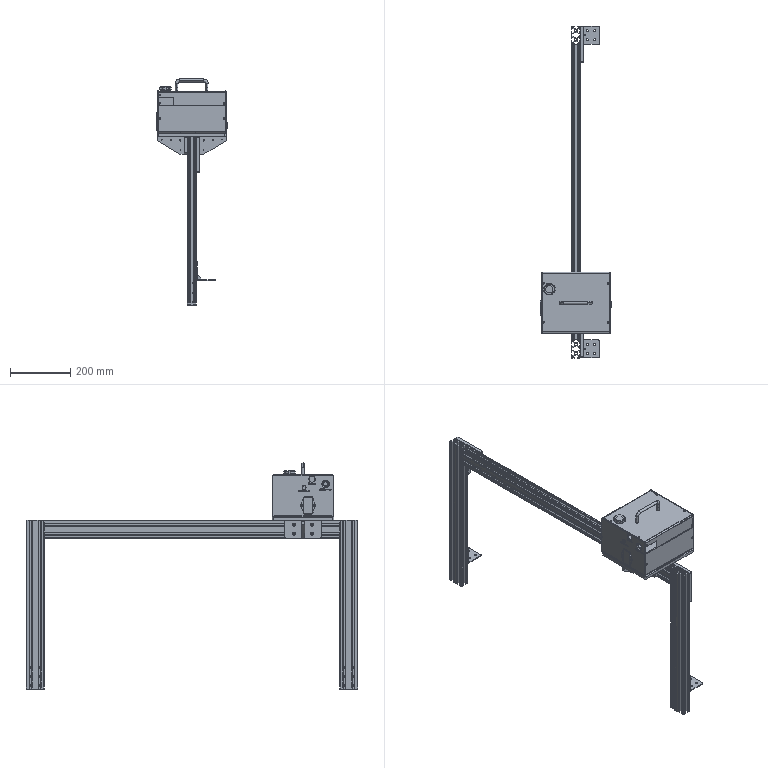Part | SolidWorks | features InContextFeatHolder 6 | 25 solids | 3533 faces | volume 2657898 mm3 | plane 1829 | spline 872 | cylinder 608 | cone 224 | commonest cylinder face diameters 6.6 x144 11 x100 10 x65 5.5 x40 3.4 x36 4.2 x36